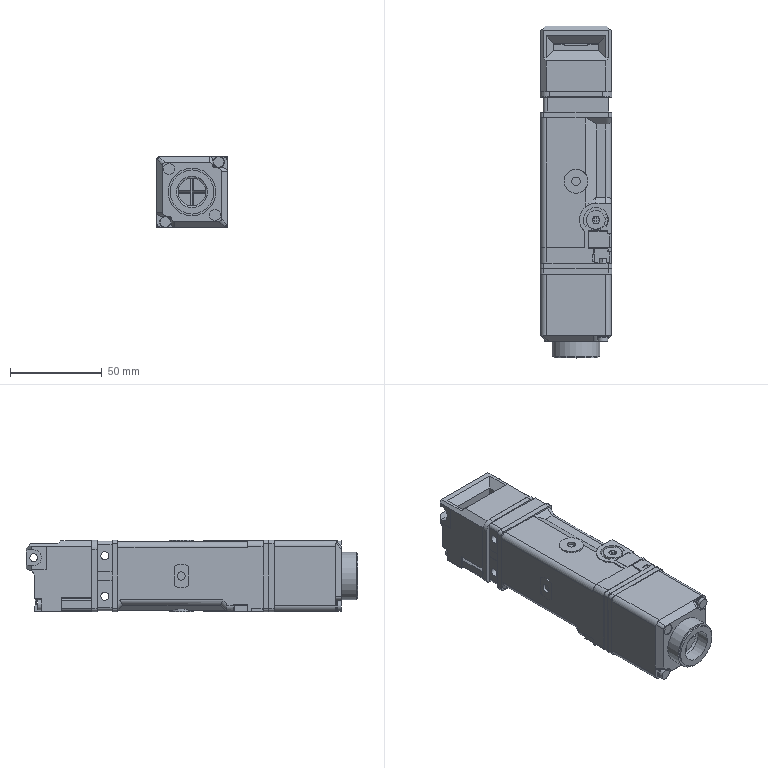Part | NX | 3 solids | 561 faces | box 39 x 180.9 x 39.045 mm | volume 232622 mm3 | plane 453 | cylinder 104 | spline 2 | cone 1 | torus 1 | commonest cylinder face diameters 4 x24 6 x19 13 x8 4.3 x7 7.4 x6 7.6 x6